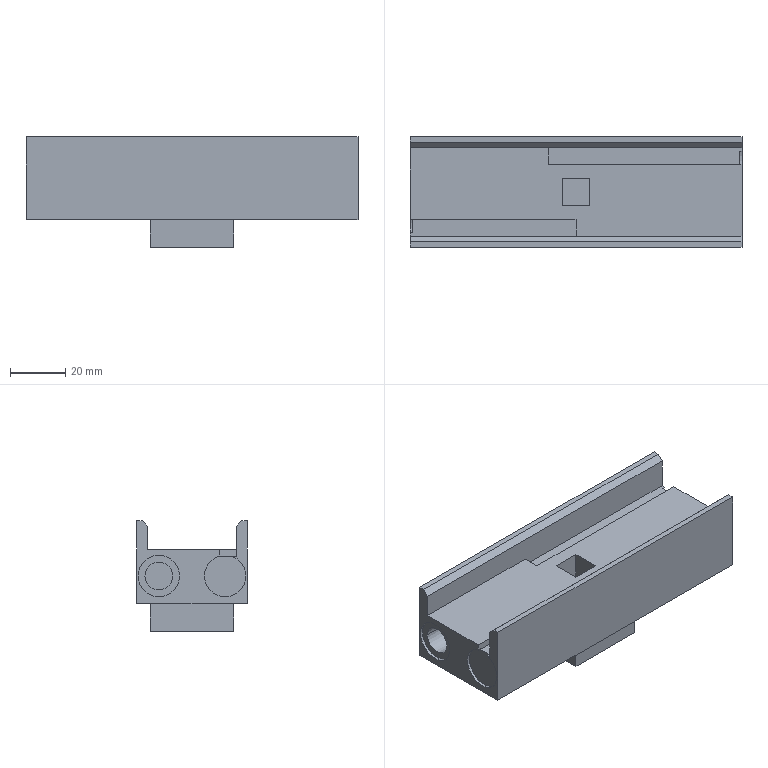Part | SolidWorks | features ICE 7, Chamfer 1, Extrusion 1, MirrorPattern 1 | 1 solid | 48 faces | box 120 x 40 x 40 mm | volume 99907 mm3 | plane 34 | cylinder 14 | commonest cylinder face diameters 15 x10 10 x4
STEP:
#1=CARTESIAN_POINT('',(-4.,17.,10.));
#2=VERTEX_POINT('',#1);
#3=CARTESIAN_POINT('',(-4.,7.,10.));
#4=VERTEX_POINT('',#3);
#5=CARTESIAN_POINT('',(-4.,12.,10.));
#6=DIRECTION('',(-1.,0.,0.));
#7=DIRECTION('',(0.,-1.,0.));
#8=AXIS2_PLACEMENT_3D('',#5,#6,#7);
#9=CIRCLE('',#8,5.);
#10=EDGE_CURVE('',#2,#4,#9,.T.);
#11=ORIENTED_EDGE('',*,*,#10,.F.);
#12=CARTESIAN_POINT('',(-59.,17.,10.));
#13=VERTEX_POINT('',#12);
#14=CARTESIAN_POINT('',(-4.,17.,10.));
#15=DIRECTION('',(-1.,0.,0.));
#16=VECTOR('',#15,1000.);
#17=LINE('',#14,#16);
#18=EDGE_CURVE('',#2,#13,#17,.T.);
#19=ORIENTED_EDGE('',*,*,#18,.T.);
#20=CARTESIAN_POINT('',(-59.,7.,10.));
#21=VERTEX_POINT('',#20);
#22=CARTESIAN_POINT('',(-59.,12.,10.));
#23=DIRECTION('',(-1.,0.,0.));
#24=DIRECTION('',(0.,-1.,0.));
#25=AXIS2_PLACEMENT_3D('',#22,#23,#24);
#26=CIRCLE('',#25,5.);
#27=EDGE_CURVE('',#13,#21,#26,.T.);
#28=ORIENTED_EDGE('',*,*,#27,.T.);
#29=CARTESIAN_POINT('',(-4.,7.,10.));
#30=DIRECTION('',(-1.,0.,0.));
#31=VECTOR('',#30,1000.);
#32=LINE('',#29,#31);
#33=EDGE_CURVE('',#4,#21,#32,.T.);
#34=ORIENTED_EDGE('',*,*,#33,.F.);
#35=EDGE_LOOP('',(#11,#19,#28,#34));
#36=FACE_OUTER_BOUND('',#35,.T.);
#37=CARTESIAN_POINT('',(-4.,12.,10.));
#38=DIRECTION('',(-1.,0.,0.));
#39=DIRECTION('',(0.,-1.,0.));
#40=AXIS2_PLACEMENT_3D('',#37,#38,#39);
#41=CYLINDRICAL_SURFACE('',#40,5.);
#42=ADVANCED_FACE('',(#36),#41,.F.);
#43=CARTESIAN_POINT('',(-59.,4.5,10.));
#44=VERTEX_POINT('',#43);
#45=CARTESIAN_POINT('',(-59.,19.5,10.));
#46=VERTEX_POINT('',#45);
#47=CARTESIAN_POINT('',(-59.,12.,10.));
#48=DIRECTION('',(1.,0.,0.));
#49=DIRECTION('',(0.,1.,0.));
#50=AXIS2_PLACEMENT_3D('',#47,#48,#49);
#51=CIRCLE('',#50,7.5);
#52=EDGE_CURVE('',#44,#46,#51,.T.);
#53=ORIENTED_EDGE('',*,*,#52,.T.);
#54=CARTESIAN_POINT('',(-60.,19.5,10.));
#55=VERTEX_POINT('',#54);
#56=CARTESIAN_POINT('',(-59.,19.5,10.));
#57=DIRECTION('',(-1.,0.,0.));
#58=VECTOR('',#57,1000.);
#59=LINE('',#56,#58);
#60=EDGE_CURVE('',#46,#55,#59,.T.);
#61=ORIENTED_EDGE('',*,*,#60,.T.);
#62=CARTESIAN_POINT('',(-60.,4.5,10.));
#63=VERTEX_POINT('',#62);
#64=CARTESIAN_POINT('',(-60.,12.,10.));
#65=DIRECTION('',(1.,0.,0.));
#66=DIRECTION('',(0.,1.,0.));
#67=AXIS2_PLACEMENT_3D('',#64,#65,#66);
#68=CIRCLE('',#67,7.5);
#69=EDGE_CURVE('',#63,#55,#68,.T.);
#70=ORIENTED_EDGE('',*,*,#69,.F.);
#71=CARTESIAN_POINT('',(-59.,4.5,10.));
#72=DIRECTION('',(-1.,0.,0.));
#73=VECTOR('',#72,1000.);
#74=LINE('',#71,#73);
#75=EDGE_CURVE('',#44,#63,#74,.T.);
#76=ORIENTED_EDGE('',*,*,#75,.F.);
#77=EDGE_LOOP('',(#53,#61,#70,#76));
#78=FACE_OUTER_BOUND('',#77,.T.);
#79=CARTESIAN_POINT('',(-59.,12.,10.));
#80=DIRECTION('',(-1.,0.,0.));
#81=DIRECTION('',(0.,-1.,0.));
#82=AXIS2_PLACEMENT_3D('',#79,#80,#81);
#83=CYLINDRICAL_SURFACE('',#82,7.5);
#84=ADVANCED_FACE('',(#78),#83,.F.);
#85=CARTESIAN_POINT('',(-59.,-19.5,10.));
#86=VERTEX_POINT('',#85);
#87=CARTESIAN_POINT('',(-59.,-4.5,10.));
#88=VERTEX_POINT('',#87);
#89=CARTESIAN_POINT('',(-59.,-12.,10.));
#90=DIRECTION('',(1.,0.,0.));
#91=DIRECTION('',(0.,1.,0.));
#92=AXIS2_PLACEMENT_3D('',#89,#90,#91);
#93=CIRCLE('',#92,7.5);
#94=EDGE_CURVE('',#86,#88,#93,.T.);
#95=ORIENTED_EDGE('',*,*,#94,.T.);
#96=CARTESIAN_POINT('',(-60.,-4.5,10.));
#97=VERTEX_POINT('',#96);
#98=CARTESIAN_POINT('',(-59.,-4.5,10.));
#99=DIRECTION('',(-1.,0.,0.));
#100=VECTOR('',#99,1000.);
#101=LINE('',#98,#100);
#102=EDGE_CURVE('',#88,#97,#101,.T.);
#103=ORIENTED_EDGE('',*,*,#102,.T.);
#104=CARTESIAN_POINT('',(-60.,-19.5,10.));
#105=VERTEX_POINT('',#104);
#106=CARTESIAN_POINT('',(-60.,-12.,10.));
#107=DIRECTION('',(1.,0.,0.));
#108=DIRECTION('',(0.,1.,0.));
#109=AXIS2_PLACEMENT_3D('',#106,#107,#108);
#110=CIRCLE('',#109,7.5);
#111=EDGE_CURVE('',#105,#97,#110,.T.);
#112=ORIENTED_EDGE('',*,*,#111,.F.);
#113=CARTESIAN_POINT('',(-59.,-19.5,10.));
#114=DIRECTION('',(-1.,0.,0.));
#115=VECTOR('',#114,1000.);
#116=LINE('',#113,#115);
#117=EDGE_CURVE('',#86,#105,#116,.T.);
#118=ORIENTED_EDGE('',*,*,#117,.F.);
#119=EDGE_LOOP('',(#95,#103,#112,#118));
#120=FACE_OUTER_BOUND('',#119,.T.);
#121=CARTESIAN_POINT('',(-59.,-12.,10.));
#122=DIRECTION('',(-1.,0.,0.));
#123=DIRECTION('',(0.,-1.,0.));
#124=AXIS2_PLACEMENT_3D('',#121,#122,#123);
#125=CYLINDRICAL_SURFACE('',#124,7.5);
#126=ADVANCED_FACE('',(#120),#125,.F.);
#127=CARTESIAN_POINT('',(-59.,-14.693,17.));
#128=VERTEX_POINT('',#127);
#129=CARTESIAN_POINT('',(-59.,-12.,10.));
#130=DIRECTION('',(1.,0.,0.));
#131=DIRECTION('',(0.,1.,0.));
#132=AXIS2_PLACEMENT_3D('',#129,#130,#131);
#133=CIRCLE('',#132,7.5);
#134=EDGE_CURVE('',#128,#86,#133,.T.);
#135=ORIENTED_EDGE('',*,*,#134,.T.);
#136=ORIENTED_EDGE('',*,*,#117,.T.);
#137=CARTESIAN_POINT('',(-60.,-14.693,17.));
#138=VERTEX_POINT('',#137);
#139=CARTESIAN_POINT('',(-60.,-12.,10.));
#140=DIRECTION('',(1.,0.,0.));
#141=DIRECTION('',(0.,1.,0.));
#142=AXIS2_PLACEMENT_3D('',#139,#140,#141);
#143=CIRCLE('',#142,7.5);
#144=EDGE_CURVE('',#138,#105,#143,.T.);
#145=ORIENTED_EDGE('',*,*,#144,.F.);
#146=CARTESIAN_POINT('',(-59.,-14.693,17.));
#147=DIRECTION('',(1.,0.,0.));
#148=VECTOR('',#147,1000.);
#149=LINE('',#146,#148);
#150=EDGE_CURVE('',#138,#128,#149,.T.);
#151=ORIENTED_EDGE('',*,*,#150,.T.);
#152=EDGE_LOOP('',(#135,#136,#145,#151));
#153=FACE_OUTER_BOUND('',#152,.T.);
#154=CARTESIAN_POINT('',(-59.,-12.,10.));
#155=DIRECTION('',(-1.,0.,0.));
#156=DIRECTION('',(0.,-1.,0.));
#157=AXIS2_PLACEMENT_3D('',#154,#155,#156);
#158=CYLINDRICAL_SURFACE('',#157,7.5);
#159=ADVANCED_FACE('',(#153),#158,.F.);
#160=CARTESIAN_POINT('',(4.,-17.,10.));
#161=VERTEX_POINT('',#160);
#162=CARTESIAN_POINT('',(4.,-7.,10.));
#163=VERTEX_POINT('',#162);
#164=CARTESIAN_POINT('',(4.,-12.,10.));
#165=DIRECTION('',(1.,0.,0.));
#166=DIRECTION('',(0.,1.,0.));
#167=AXIS2_PLACEMENT_3D('',#164,#165,#166);
#168=CIRCLE('',#167,5.);
#169=EDGE_CURVE('',#161,#163,#168,.T.);
#170=ORIENTED_EDGE('',*,*,#169,.F.);
#171=CARTESIAN_POINT('',(59.,-17.,10.));
#172=VERTEX_POINT('',#171);
#173=CARTESIAN_POINT('',(4.,-17.,10.));
#174=DIRECTION('',(1.,0.,0.));
#175=VECTOR('',#174,1000.);
#176=LINE('',#173,#175);
#177=EDGE_CURVE('',#161,#172,#176,.T.);
#178=ORIENTED_EDGE('',*,*,#177,.T.);
#179=CARTESIAN_POINT('',(59.,-7.,10.));
#180=VERTEX_POINT('',#179);
#181=CARTESIAN_POINT('',(59.,-12.,10.));
#182=DIRECTION('',(1.,0.,0.));
#183=DIRECTION('',(0.,1.,0.));
#184=AXIS2_PLACEMENT_3D('',#181,#182,#183);
#185=CIRCLE('',#184,5.);
#186=EDGE_CURVE('',#172,#180,#185,.T.);
#187=ORIENTED_EDGE('',*,*,#186,.T.);
#188=CARTESIAN_POINT('',(4.,-7.,10.));
#189=DIRECTION('',(1.,0.,0.));
#190=VECTOR('',#189,1000.);
#191=LINE('',#188,#190);
#192=EDGE_CURVE('',#163,#180,#191,.T.);
#193=ORIENTED_EDGE('',*,*,#192,.F.);
#194=EDGE_LOOP('',(#170,#178,#187,#193));
#195=FACE_OUTER_BOUND('',#194,.T.);
#196=CARTESIAN_POINT('',(4.,-12.,10.));
#197=DIRECTION('',(1.,0.,0.));
#198=DIRECTION('',(0.,1.,0.));
#199=AXIS2_PLACEMENT_3D('',#196,#197,#198);
#200=CYLINDRICAL_SURFACE('',#199,5.);
#201=ADVANCED_FACE('',(#195),#200,.F.);
#202=CARTESIAN_POINT('',(59.,4.5,10.));
#203=VERTEX_POINT('',#202);
#204=CARTESIAN_POINT('',(59.,19.5,10.));
#205=VERTEX_POINT('',#204);
#206=CARTESIAN_POINT('',(59.,12.,10.));
#207=DIRECTION('',(1.,0.,0.));
#208=DIRECTION('',(0.,1.,0.));
#209=AXIS2_PLACEMENT_3D('',#206,#207,#208);
#210=CIRCLE('',#209,7.5);
#211=EDGE_CURVE('',#203,#205,#210,.T.);
#212=ORIENTED_EDGE('',*,*,#211,.F.);
#213=CARTESIAN_POINT('',(60.,4.5,10.));
#214=VERTEX_POINT('',#213);
#215=CARTESIAN_POINT('',(59.,4.5,10.));
#216=DIRECTION('',(1.,0.,0.));
#217=VECTOR('',#216,1000.);
#218=LINE('',#215,#217);
#219=EDGE_CURVE('',#203,#214,#218,.T.);
#220=ORIENTED_EDGE('',*,*,#219,.T.);
#221=CARTESIAN_POINT('',(60.,19.5,10.));
#222=VERTEX_POINT('',#221);
#223=CARTESIAN_POINT('',(60.,12.,10.));
#224=DIRECTION('',(1.,0.,0.));
#225=DIRECTION('',(0.,1.,0.));
#226=AXIS2_PLACEMENT_3D('',#223,#224,#225);
#227=CIRCLE('',#226,7.5);
#228=EDGE_CURVE('',#214,#222,#227,.T.);
#229=ORIENTED_EDGE('',*,*,#228,.T.);
#230=CARTESIAN_POINT('',(59.,19.5,10.));
#231=DIRECTION('',(1.,0.,0.));
#232=VECTOR('',#231,1000.);
#233=LINE('',#230,#232);
#234=EDGE_CURVE('',#205,#222,#233,.T.);
#235=ORIENTED_EDGE('',*,*,#234,.F.);
#236=EDGE_LOOP('',(#212,#220,#229,#235));
#237=FACE_OUTER_BOUND('',#236,.T.);
#238=CARTESIAN_POINT('',(59.,12.,10.));
#239=DIRECTION('',(1.,0.,0.));
#240=DIRECTION('',(0.,1.,0.));
#241=AXIS2_PLACEMENT_3D('',#238,#239,#240);
#242=CYLINDRICAL_SURFACE('',#241,7.5);
#243=ADVANCED_FACE('',(#237),#242,.F.);
#244=CARTESIAN_POINT('',(59.,14.693,17.));
#245=VERTEX_POINT('',#244);
#246=CARTESIAN_POINT('',(59.,12.,10.));
#247=DIRECTION('',(1.,0.,0.));
#248=DIRECTION('',(0.,1.,0.));
#249=AXIS2_PLACEMENT_3D('',#246,#247,#248);
#250=CIRCLE('',#249,7.5);
#251=EDGE_CURVE('',#205,#245,#250,.T.);
#252=ORIENTED_EDGE('',*,*,#251,.F.);
#253=ORIENTED_EDGE('',*,*,#234,.T.);
#254=CARTESIAN_POINT('',(60.,14.693,17.));
#255=VERTEX_POINT('',#254);
#256=CARTESIAN_POINT('',(60.,12.,10.));
#257=DIRECTION('',(1.,0.,0.));
#258=DIRECTION('',(0.,1.,0.));
#259=AXIS2_PLACEMENT_3D('',#256,#257,#258);
#260=CIRCLE('',#259,7.5);
#261=EDGE_CURVE('',#222,#255,#260,.T.);
#262=ORIENTED_EDGE('',*,*,#261,.T.);
#263=CARTESIAN_POINT('',(59.,14.693,17.));
#264=DIRECTION('',(1.,0.,0.));
#265=VECTOR('',#264,1000.);
#266=LINE('',#263,#265);
#267=EDGE_CURVE('',#245,#255,#266,.T.);
#268=ORIENTED_EDGE('',*,*,#267,.F.);
#269=EDGE_LOOP('',(#252,#253,#262,#268));
#270=FACE_OUTER_BOUND('',#269,.T.);
#271=CARTESIAN_POINT('',(59.,12.,10.));
#272=DIRECTION('',(1.,0.,0.));
#273=DIRECTION('',(0.,1.,0.));
#274=AXIS2_PLACEMENT_3D('',#271,#272,#273);
#275=CYLINDRICAL_SURFACE('',#274,7.5);
#276=ADVANCED_FACE('',(#270),#275,.F.);
#277=CARTESIAN_POINT('',(59.,-19.5,10.));
#278=VERTEX_POINT('',#277);
#279=CARTESIAN_POINT('',(59.,-4.5,10.));
#280=VERTEX_POINT('',#279);
#281=CARTESIAN_POINT('',(59.,-12.,10.));
#282=DIRECTION('',(1.,0.,0.));
#283=DIRECTION('',(0.,1.,0.));
#284=AXIS2_PLACEMENT_3D('',#281,#282,#283);
#285=CIRCLE('',#284,7.5);
#286=EDGE_CURVE('',#278,#280,#285,.T.);
#287=ORIENTED_EDGE('',*,*,#286,.F.);
#288=CARTESIAN_POINT('',(60.,-19.5,10.));
#289=VERTEX_POINT('',#288);
#290=CARTESIAN_POINT('',(59.,-19.5,10.));
#291=DIRECTION('',(1.,0.,0.));
#292=VECTOR('',#291,1000.);
#293=LINE('',#290,#292);
#294=EDGE_CURVE('',#278,#289,#293,.T.);
#295=ORIENTED_EDGE('',*,*,#294,.T.);
#296=CARTESIAN_POINT('',(60.,-4.5,10.));
#297=VERTEX_POINT('',#296);
#298=CARTESIAN_POINT('',(60.,-12.,10.));
#299=DIRECTION('',(1.,0.,0.));
#300=DIRECTION('',(0.,1.,0.));
#301=AXIS2_PLACEMENT_3D('',#298,#299,#300);
#302=CIRCLE('',#301,7.5);
#303=EDGE_CURVE('',#289,#297,#302,.T.);
#304=ORIENTED_EDGE('',*,*,#303,.T.);
#305=CARTESIAN_POINT('',(59.,-4.5,10.));
#306=DIRECTION('',(1.,0.,0.));
#307=VECTOR('',#306,1000.);
#308=LINE('',#305,#307);
#309=EDGE_CURVE('',#280,#297,#308,.T.);
#310=ORIENTED_EDGE('',*,*,#309,.F.);
#311=EDGE_LOOP('',(#287,#295,#304,#310));
#312=FACE_OUTER_BOUND('',#311,.T.);
#313=CARTESIAN_POINT('',(59.,-12.,10.));
#314=DIRECTION('',(1.,0.,0.));
#315=DIRECTION('',(0.,1.,0.));
#316=AXIS2_PLACEMENT_3D('',#313,#314,#315);
#317=CYLINDRICAL_SURFACE('',#316,7.5);
#318=ADVANCED_FACE('',(#312),#317,.F.);
#319=ORIENTED_EDGE('',*,*,#150,.F.);
#320=CARTESIAN_POINT('',(-60.,-16.,17.));
#321=VERTEX_POINT('',#320);
#322=CARTESIAN_POINT('',(-60.,-16.,17.));
#323=DIRECTION('',(0.,-1.,0.));
#324=VECTOR('',#323,1000.);
#325=LINE('',#322,#324);
#326=EDGE_CURVE('',#138,#321,#325,.T.);
#327=ORIENTED_EDGE('',*,*,#326,.T.);
#328=CARTESIAN_POINT('',(0.,-16.,17.));
#329=VERTEX_POINT('',#328);
#330=CARTESIAN_POINT('',(0.,-16.,17.));
#331=DIRECTION('',(-1.,0.,0.));
#332=VECTOR('',#331,1000.);
#333=LINE('',#330,#332);
#334=EDGE_CURVE('',#329,#321,#333,.T.);
#335=ORIENTED_EDGE('',*,*,#334,.F.);
#336=CARTESIAN_POINT('',(0.,-10.,17.));
#337=VERTEX_POINT('',#336);
#338=CARTESIAN_POINT('',(0.,-16.,17.));
#339=DIRECTION('',(0.,-1.,0.));
#340=VECTOR('',#339,1000.);
#341=LINE('',#338,#340);
#342=EDGE_CURVE('',#337,#329,#341,.T.);
#343=ORIENTED_EDGE('',*,*,#342,.F.);
#344=CARTESIAN_POINT('',(-59.,-10.,17.));
#345=VERTEX_POINT('',#344);
#346=CARTESIAN_POINT('',(0.,-10.,17.));
#347=DIRECTION('',(-1.,0.,0.));
#348=VECTOR('',#347,1000.);
#349=LINE('',#346,#348);
#350=EDGE_CURVE('',#337,#345,#349,.T.);
#351=ORIENTED_EDGE('',*,*,#350,.T.);
#352=CARTESIAN_POINT('',(-59.,-16.,17.));
#353=DIRECTION('',(0.,1.,0.));
#354=VECTOR('',#353,1000.);
#355=LINE('',#352,#354);
#356=EDGE_CURVE('',#128,#345,#355,.T.);
#357=ORIENTED_EDGE('',*,*,#356,.F.);
#358=EDGE_LOOP('',(#319,#327,#335,#343,#351,#357));
#359=FACE_OUTER_BOUND('',#358,.T.);
#360=CARTESIAN_POINT('',(0.,-16.,17.));
#361=DIRECTION('',(0.,0.,-1.));
#362=DIRECTION('',(-1.,0.,0.));
#363=AXIS2_PLACEMENT_3D('',#360,#361,#362);
#364=PLANE('',#363);
#365=ADVANCED_FACE('',(#359),#364,.F.);
#366=CARTESIAN_POINT('',(-59.,-10.,17.228));
#367=VERTEX_POINT('',#366);
#368=CARTESIAN_POINT('',(-60.,-10.,17.228));
#369=VERTEX_POINT('',#368);
#370=CARTESIAN_POINT('',(-59.,-10.,17.228));
#371=DIRECTION('',(-1.,0.,0.));
#372=VECTOR('',#371,1000.);
#373=LINE('',#370,#372);
#374=EDGE_CURVE('',#367,#369,#373,.T.);
#375=ORIENTED_EDGE('',*,*,#374,.F.);
#376=CARTESIAN_POINT('',(-59.,-10.,19.5));
#377=DIRECTION('',(0.,0.,1.));
#378=VECTOR('',#377,1000.);
#379=LINE('',#376,#378);
#380=EDGE_CURVE('',#345,#367,#379,.T.);
#381=ORIENTED_EDGE('',*,*,#380,.F.);
#382=ORIENTED_EDGE('',*,*,#350,.F.);
#383=CARTESIAN_POINT('',(0.,-10.,19.5));
#384=VERTEX_POINT('',#383);
#385=CARTESIAN_POINT('',(0.,-10.,19.5));
#386=DIRECTION('',(0.,0.,-1.));
#387=VECTOR('',#386,1000.);
#388=LINE('',#385,#387);
#389=EDGE_CURVE('',#384,#337,#388,.T.);
#390=ORIENTED_EDGE('',*,*,#389,.F.);
#391=CARTESIAN_POINT('',(-60.,-10.,19.5));
#392=VERTEX_POINT('',#391);
#393=CARTESIAN_POINT('',(0.,-10.,19.5));
#394=DIRECTION('',(-1.,0.,0.));
#395=VECTOR('',#394,1000.);
#396=LINE('',#393,#395);
#397=EDGE_CURVE('',#384,#392,#396,.T.);
#398=ORIENTED_EDGE('',*,*,#397,.T.);
#399=CARTESIAN_POINT('',(-60.,-10.,19.5));
#400=DIRECTION('',(0.,0.,-1.));
#401=VECTOR('',#400,1000.);
#402=LINE('',#399,#401);
#403=EDGE_CURVE('',#392,#369,#402,.T.);
#404=ORIENTED_EDGE('',*,*,#403,.T.);
#405=EDGE_LOOP('',(#375,#381,#382,#390,#398,#404));
#406=FACE_OUTER_BOUND('',#405,.T.);
#407=CARTESIAN_POINT('',(0.,-10.,19.5));
#408=DIRECTION('',(0.,1.,0.));
#409=DIRECTION('',(-1.,0.,0.));
#410=AXIS2_PLACEMENT_3D('',#407,#408,#409);
#411=PLANE('',#410);
#412=ADVANCED_FACE('',(#406),#411,.F.);
#413=CARTESIAN_POINT('',(60.,-20.,0.));
#414=VERTEX_POINT('',#413);
#415=CARTESIAN_POINT('',(60.,20.,0.));
#416=VERTEX_POINT('',#415);
#417=CARTESIAN_POINT('',(60.,20.,0.));
#418=DIRECTION('',(0.,1.,0.));
#419=VECTOR('',#418,1000.);
#420=LINE('',#417,#419);
#421=EDGE_CURVE('',#414,#416,#420,.T.);
#422=ORIENTED_EDGE('',*,*,#421,.F.);
#423=CARTESIAN_POINT('',(-60.,-20.,0.));
#424=VERTEX_POINT('',#423);
#425=CARTESIAN_POINT('',(-60.,-20.,0.));
#426=DIRECTION('',(1.,0.,0.));
#427=VECTOR('',#426,1000.);
#428=LINE('',#425,#427);
#429=EDGE_CURVE('',#424,#414,#428,.T.);
#430=ORIENTED_EDGE('',*,*,#429,.F.);
#431=CARTESIAN_POINT('',(-60.,20.,0.));
#432=VERTEX_POINT('',#431);
#433=CARTESIAN_POINT('',(-60.,20.,0.));
#434=DIRECTION('',(0.,-1.,0.));
#435=VECTOR('',#434,1000.);
#436=LINE('',#433,#435);
#437=EDGE_CURVE('',#432,#424,#436,.T.);
#438=ORIENTED_EDGE('',*,*,#437,.F.);
#439=CARTESIAN_POINT('',(-60.,20.,0.));
#440=DIRECTION('',(-1.,0.,0.));
#441=VECTOR('',#440,1000.);
#442=LINE('',#439,#441);
#443=EDGE_CURVE('',#416,#432,#442,.T.);
#444=ORIENTED_EDGE('',*,*,#443,.F.);
#445=EDGE_LOOP('',(#422,#430,#438,#444));
#446=FACE_OUTER_BOUND('',#445,.T.);
#447=CARTESIAN_POINT('',(-15.,-15.,0.));
#448=VERTEX_POINT('',#447);
#449=CARTESIAN_POINT('',(-15.,15.,0.));
#450=VERTEX_POINT('',#449);
#451=CARTESIAN_POINT('',(-15.,15.,0.));
#452=DIRECTION('',(0.,1.,0.));
#453=VECTOR('',#452,1000.);
#454=LINE('',#451,#453);
#455=EDGE_CURVE('',#448,#450,#454,.T.);
#456=ORIENTED_EDGE('',*,*,#455,.F.);
#457=CARTESIAN_POINT('',(15.,-15.,0.));
#458=VERTEX_POINT('',#457);
#459=CARTESIAN_POINT('',(15.,-15.,0.));
#460=DIRECTION('',(-1.,0.,0.));
#461=VECTOR('',#460,1000.);
#462=LINE('',#459,#461);
#463=EDGE_CURVE('',#458,#448,#462,.T.);
#464=ORIENTED_EDGE('',*,*,#463,.F.);
#465=CARTESIAN_POINT('',(15.,15.,0.));
#466=VERTEX_POINT('',#465);
#467=CARTESIAN_POINT('',(15.,15.,0.));
#468=DIRECTION('',(0.,-1.,0.));
#469=VECTOR('',#468,1000.);
#470=LINE('',#467,#469);
#471=EDGE_CURVE('',#466,#458,#470,.T.);
#472=ORIENTED_EDGE('',*,*,#471,.F.);
#473=CARTESIAN_POINT('',(15.,15.,0.));
#474=DIRECTION('',(1.,0.,0.));
#475=VECTOR('',#474,1000.);
#476=LINE('',#473,#475);
#477=EDGE_CURVE('',#450,#466,#476,.T.);
#478=ORIENTED_EDGE('',*,*,#477,.F.);
#479=EDGE_LOOP('',(#456,#464,#472,#478));
#480=FACE_BOUND('',#479,.T.);
#481=CARTESIAN_POINT('',(0.,0.,0.));
#482=DIRECTION('',(0.,0.,1.));
#483=DIRECTION('',(1.,0.,0.));
#484=AXIS2_PLACEMENT_3D('',#481,#482,#483);
#485=PLANE('',#484);
#486=ADVANCED_FACE('',(#446,#480),#485,.F.);
#487=CARTESIAN_POINT('',(60.,-20.,30.));
#488=VERTEX_POINT('',#487);
#489=CARTESIAN_POINT('',(60.,-18.,30.));
#490=VERTEX_POINT('',#489);
#491=CARTESIAN_POINT('',(60.,20.,30.));
#492=DIRECTION('',(0.,1.,0.));
#493=VECTOR('',#492,1000.);
#494=LINE('',#491,#493);
#495=EDGE_CURVE('',#488,#490,#494,.T.);
#496=ORIENTED_EDGE('',*,*,#495,.T.);
#497=CARTESIAN_POINT('',(-60.,-18.,30.));
#498=VERTEX_POINT('',#497);
#499=CARTESIAN_POINT('',(-60.,-18.,30.));
#500=DIRECTION('',(-1.,0.,0.));
#501=VECTOR('',#500,1000.);
#502=LINE('',#499,#501);
#503=EDGE_CURVE('',#490,#498,#502,.T.);
#504=ORIENTED_EDGE('',*,*,#503,.T.);
#505=CARTESIAN_POINT('',(-60.,-20.,30.));
#506=VERTEX_POINT('',#505);
#507=CARTESIAN_POINT('',(-60.,20.,30.));
#508=DIRECTION('',(0.,-1.,0.));
#509=VECTOR('',#508,1000.);
#510=LINE('',#507,#509);
#511=EDGE_CURVE('',#498,#506,#510,.T.);
#512=ORIENTED_EDGE('',*,*,#511,.T.);
#513=CARTESIAN_POINT('',(-60.,-20.,30.));
#514=DIRECTION('',(1.,0.,0.));
#515=VECTOR('',#514,1000.);
#516=LINE('',#513,#515);
#517=EDGE_CURVE('',#506,#488,#516,.T.);
#518=ORIENTED_EDGE('',*,*,#517,.T.);
#519=EDGE_LOOP('',(#496,#504,#512,#518));
#520=FACE_OUTER_BOUND('',#519,.T.);
#521=CARTESIAN_POINT('',(0.,0.,30.));
#522=DIRECTION('',(0.,0.,1.));
#523=DIRECTION('',(1.,0.,0.));
#524=AXIS2_PLACEMENT_3D('',#521,#522,#523);
#525=PLANE('',#524);
#526=ADVANCED_FACE('',(#520),#525,.T.);
#527=CARTESIAN_POINT('',(60.,-12.,10.));
#528=DIRECTION('',(1.,0.,0.));
#529=DIRECTION('',(0.,1.,0.));
#530=AXIS2_PLACEMENT_3D('',#527,#528,#529);
#531=CIRCLE('',#530,7.5);
#532=EDGE_CURVE('',#297,#289,#531,.T.);
#533=ORIENTED_EDGE('',*,*,#532,.F.);
#534=ORIENTED_EDGE('',*,*,#303,.F.);
#535=EDGE_LOOP('',(#533,#534));
#536=FACE_BOUND('',#535,.T.);
#537=CARTESIAN_POINT('',(60.,16.,17.));
#538=VERTEX_POINT('',#537);
#539=CARTESIAN_POINT('',(60.,16.,17.));
#540=DIRECTION('',(0.,1.,0.));
#541=VECTOR('',#540,1000.);
#542=LINE('',#539,#541);
#543=EDGE_CURVE('',#255,#538,#542,.T.);
#544=ORIENTED_EDGE('',*,*,#543,.F.);
#545=ORIENTED_EDGE('',*,*,#261,.F.);
#546=ORIENTED_EDGE('',*,*,#228,.F.);
#547=CARTESIAN_POINT('',(60.,10.,17.228));
#548=VERTEX_POINT('',#547);
#549=CARTESIAN_POINT('',(60.,12.,10.));
#550=DIRECTION('',(1.,0.,0.));
#551=DIRECTION('',(0.,1.,0.));
#552=AXIS2_PLACEMENT_3D('',#549,#550,#551);
#553=CIRCLE('',#552,7.5);
#554=EDGE_CURVE('',#548,#214,#553,.T.);
#555=ORIENTED_EDGE('',*,*,#554,.F.);
#556=CARTESIAN_POINT('',(60.,10.,19.5));
#557=VERTEX_POINT('',#556);
#558=CARTESIAN_POINT('',(60.,10.,19.5));
#559=DIRECTION('',(0.,0.,-1.));
#560=VECTOR('',#559,1000.);
#561=LINE('',#558,#560);
#562=EDGE_CURVE('',#557,#548,#561,.T.);
#563=ORIENTED_EDGE('',*,*,#562,.F.);
#564=CARTESIAN_POINT('',(60.,-16.,19.5));
#565=VERTEX_POINT('',#564);
#566=CARTESIAN_POINT('',(60.,10.,19.5));
#567=DIRECTION('',(0.,1.,0.));
#568=VECTOR('',#567,1000.);
#569=LINE('',#566,#568);
#570=EDGE_CURVE('',#565,#557,#569,.T.);
#571=ORIENTED_EDGE('',*,*,#570,.F.);
#572=CARTESIAN_POINT('',(60.,-16.,28.));
#573=VERTEX_POINT('',#572);
#574=CARTESIAN_POINT('',(60.,-16.,30.));
#575=DIRECTION('',(0.,0.,-1.));
#576=VECTOR('',#575,1000.);
#577=LINE('',#574,#576);
#578=EDGE_CURVE('',#573,#565,#577,.T.);
#579=ORIENTED_EDGE('',*,*,#578,.F.);
#580=CARTESIAN_POINT('',(60.,-16.,28.));
#581=DIRECTION('',(0.,-0.7071,0.7071));
#582=VECTOR('',#581,1000.);
#583=LINE('',#580,#582);
#584=EDGE_CURVE('',#573,#490,#583,.T.);
#585=ORIENTED_EDGE('',*,*,#584,.T.);
#586=ORIENTED_EDGE('',*,*,#495,.F.);
#587=CARTESIAN_POINT('',(60.,-20.,30.));
#588=DIRECTION('',(0.,0.,-1.));
#589=VECTOR('',#588,1000.);
#590=LINE('',#587,#589);
#591=EDGE_CURVE('',#488,#414,#590,.T.);
#592=ORIENTED_EDGE('',*,*,#591,.T.);
#593=ORIENTED_EDGE('',*,*,#421,.T.);
#594=CARTESIAN_POINT('',(60.,20.,30.));
#595=VERTEX_POINT('',#594);
#596=CARTESIAN_POINT('',(60.,20.,30.));
#597=DIRECTION('',(0.,0.,-1.));
#598=VECTOR('',#597,1000.);
#599=LINE('',#596,#598);
#600=EDGE_CURVE('',#595,#416,#599,.T.);
#601=ORIENTED_EDGE('',*,*,#600,.F.);
#602=CARTESIAN_POINT('',(60.,18.,30.));
#603=VERTEX_POINT('',#602);
#604=CARTESIAN_POINT('',(60.,20.,30.));
#605=DIRECTION('',(0.,1.,0.));
#606=VECTOR('',#605,1000.);
#607=LINE('',#604,#606);
#608=EDGE_CURVE('',#603,#595,#607,.T.);
#609=ORIENTED_EDGE('',*,*,#608,.F.);
#610=CARTESIAN_POINT('',(60.,16.,28.));
#611=VERTEX_POINT('',#610);
#612=CARTESIAN_POINT('',(60.,18.,30.));
#613=DIRECTION('',(0.,-0.7071,-0.7071));
#614=VECTOR('',#613,1000.);
#615=LINE('',#612,#614);
#616=EDGE_CURVE('',#603,#611,#615,.T.);
#617=ORIENTED_EDGE('',*,*,#616,.T.);
#618=CARTESIAN_POINT('',(60.,16.,30.));
#619=DIRECTION('',(0.,0.,1.));
#620=VECTOR('',#619,1000.);
#621=LINE('',#618,#620);
#622=EDGE_CURVE('',#538,#611,#621,.T.);
#623=ORIENTED_EDGE('',*,*,#622,.F.);
#624=EDGE_LOOP('',(#544,#545,#546,#555,#563,#571,#579,#585,#586,#592,#593,#601,#609,#617,#623));
#625=FACE_OUTER_BOUND('',#624,.T.);
#626=CARTESIAN_POINT('',(60.,20.,30.));
#627=DIRECTION('',(-1.,0.,0.));
#628=DIRECTION('',(0.,-1.,0.));
#629=AXIS2_PLACEMENT_3D('',#626,#627,#628);
#630=PLANE('',#629);
#631=ADVANCED_FACE('',(#536,#625),#630,.F.);
#632=ORIENTED_EDGE('',*,*,#443,.T.);
#633=CARTESIAN_POINT('',(-60.,20.,30.));
#634=VERTEX_POINT('',#633);
#635=CARTESIAN_POINT('',(-60.,20.,30.));
#636=DIRECTION('',(0.,0.,-1.));
#637=VECTOR('',#636,1000.);
#638=LINE('',#635,#637);
#639=EDGE_CURVE('',#634,#432,#638,.T.);
#640=ORIENTED_EDGE('',*,*,#639,.F.);
#641=CARTESIAN_POINT('',(-60.,20.,30.));
#642=DIRECTION('',(-1.,0.,0.));
#643=VECTOR('',#642,1000.);
#644=LINE('',#641,#643);
#645=EDGE_CURVE('',#595,#634,#644,.T.);
#646=ORIENTED_EDGE('',*,*,#645,.F.);
#647=ORIENTED_EDGE('',*,*,#600,.T.);
#648=EDGE_LOOP('',(#632,#640,#646,#647));
#649=FACE_OUTER_BOUND('',#648,.T.);
#650=CARTESIAN_POINT('',(-60.,20.,30.));
#651=DIRECTION('',(0.,-1.,0.));
#652=DIRECTION('',(0.,0.,-1.));
#653=AXIS2_PLACEMENT_3D('',#650,#651,#652);
#654=PLANE('',#653);
#655=ADVANCED_FACE('',(#649),#654,.F.);
#656=ORIENTED_EDGE('',*,*,#69,.T.);
#657=CARTESIAN_POINT('',(-60.,12.,10.));
#658=DIRECTION('',(1.,0.,0.));
#659=DIRECTION('',(0.,1.,0.));
#660=AXIS2_PLACEMENT_3D('',#657,#658,#659);
#661=CIRCLE('',#660,7.5);
#662=EDGE_CURVE('',#55,#63,#661,.T.);
#663=ORIENTED_EDGE('',*,*,#662,.T.);
#664=EDGE_LOOP('',(#656,#663));
#665=FACE_BOUND('',#664,.T.);
#666=ORIENTED_EDGE('',*,*,#144,.T.);
#667=ORIENTED_EDGE('',*,*,#111,.T.);
#668=CARTESIAN_POINT('',(-60.,-12.,10.));
#669=DIRECTION('',(1.,0.,0.));
#670=DIRECTION('',(0.,1.,0.));
#671=AXIS2_PLACEMENT_3D('',#668,#669,#670);
#672=CIRCLE('',#671,7.5);
#673=EDGE_CURVE('',#97,#369,#672,.T.);
#674=ORIENTED_EDGE('',*,*,#673,.T.);
#675=ORIENTED_EDGE('',*,*,#403,.F.);
#676=CARTESIAN_POINT('',(-60.,16.,19.5));
#677=VERTEX_POINT('',#676);
#678=CARTESIAN_POINT('',(-60.,16.,19.5));
#679=DIRECTION('',(0.,-1.,0.));
#680=VECTOR('',#679,1000.);
#681=LINE('',#678,#680);
#682=EDGE_CURVE('',#677,#392,#681,.T.);
#683=ORIENTED_EDGE('',*,*,#682,.F.);
#684=CARTESIAN_POINT('',(-60.,16.,28.));
#685=VERTEX_POINT('',#684);
#686=CARTESIAN_POINT('',(-60.,16.,30.));
#687=DIRECTION('',(0.,0.,-1.));
#688=VECTOR('',#687,1000.);
#689=LINE('',#686,#688);
#690=EDGE_CURVE('',#685,#677,#689,.T.);
#691=ORIENTED_EDGE('',*,*,#690,.F.);
#692=CARTESIAN_POINT('',(-60.,18.,30.));
#693=VERTEX_POINT('',#692);
#694=CARTESIAN_POINT('',(-60.,18.,30.));
#695=DIRECTION('',(0.,0.7071,0.7071));
#696=VECTOR('',#695,1000.);
#697=LINE('',#694,#696);
#698=EDGE_CURVE('',#685,#693,#697,.T.);
#699=ORIENTED_EDGE('',*,*,#698,.T.);
#700=CARTESIAN_POINT('',(-60.,20.,30.));
#701=DIRECTION('',(0.,-1.,0.));
#702=VECTOR('',#701,1000.);
#703=LINE('',#700,#702);
#704=EDGE_CURVE('',#634,#693,#703,.T.);
#705=ORIENTED_EDGE('',*,*,#704,.F.);
#706=ORIENTED_EDGE('',*,*,#639,.T.);
#707=ORIENTED_EDGE('',*,*,#437,.T.);
#708=CARTESIAN_POINT('',(-60.,-20.,30.));
#709=DIRECTION('',(0.,0.,-1.));
#710=VECTOR('',#709,1000.);
#711=LINE('',#708,#710);
#712=EDGE_CURVE('',#506,#424,#711,.T.);
#713=ORIENTED_EDGE('',*,*,#712,.F.);
#714=ORIENTED_EDGE('',*,*,#511,.F.);
#715=CARTESIAN_POINT('',(-60.,-16.,28.));
#716=VERTEX_POINT('',#715);
#717=CARTESIAN_POINT('',(-60.,-16.,28.));
#718=DIRECTION('',(0.,0.7071,-0.7071));
#719=VECTOR('',#718,1000.);
#720=LINE('',#717,#719);
#721=EDGE_CURVE('',#498,#716,#720,.T.);
#722=ORIENTED_EDGE('',*,*,#721,.T.);
#723=CARTESIAN_POINT('',(-60.,-16.,30.));
#724=DIRECTION('',(0.,0.,1.));
#725=VECTOR('',#724,1000.);
#726=LINE('',#723,#725);
#727=EDGE_CURVE('',#321,#716,#726,.T.);
#728=ORIENTED_EDGE('',*,*,#727,.F.);
#729=ORIENTED_EDGE('',*,*,#326,.F.);
#730=EDGE_LOOP('',(#666,#667,#674,#675,#683,#691,#699,#705,#706,#707,#713,#714,#722,#728,#729));
#731=FACE_OUTER_BOUND('',#730,.T.);
#732=CARTESIAN_POINT('',(-60.,20.,30.));
#733=DIRECTION('',(1.,0.,0.));
#734=DIRECTION('',(0.,1.,0.));
#735=AXIS2_PLACEMENT_3D('',#732,#733,#734);
#736=PLANE('',#735);
#737=ADVANCED_FACE('',(#665,#731),#736,.F.);
#738=ORIENTED_EDGE('',*,*,#429,.T.);
#739=ORIENTED_EDGE('',*,*,#591,.F.);
#740=ORIENTED_EDGE('',*,*,#517,.F.);
#741=ORIENTED_EDGE('',*,*,#712,.T.);
#742=EDGE_LOOP('',(#738,#739,#740,#741));
#743=FACE_OUTER_BOUND('',#742,.T.);
#744=CARTESIAN_POINT('',(-60.,-20.,30.));
#745=DIRECTION('',(0.,1.,0.));
#746=DIRECTION('',(0.,0.,1.));
#747=AXIS2_PLACEMENT_3D('',#744,#745,#746);
#748=PLANE('',#747);
#749=ADVANCED_FACE('',(#743),#748,.F.);
#750=ORIENTED_EDGE('',*,*,#704,.T.);
#751=CARTESIAN_POINT('',(60.,18.,30.));
#752=DIRECTION('',(1.,0.,0.));
#753=VECTOR('',#752,1000.);
#754=LINE('',#751,#753);
#755=EDGE_CURVE('',#693,#603,#754,.T.);
#756=ORIENTED_EDGE('',*,*,#755,.T.);
#757=ORIENTED_EDGE('',*,*,#608,.T.);
#758=ORIENTED_EDGE('',*,*,#645,.T.);
#759=EDGE_LOOP('',(#750,#756,#757,#758));
#760=FACE_OUTER_BOUND('',#759,.T.);
#761=CARTESIAN_POINT('',(0.,0.,30.));
#762=DIRECTION('',(0.,0.,1.));
#763=DIRECTION('',(1.,0.,0.));
#764=AXIS2_PLACEMENT_3D('',#761,#762,#763);
#765=PLANE('',#764);
#766=ADVANCED_FACE('',(#760),#765,.T.);
#767=ORIENTED_EDGE('',*,*,#622,.T.);
#768=CARTESIAN_POINT('',(-60.,16.,28.));
#769=DIRECTION('',(-1.,0.,0.));
#770=VECTOR('',#769,1000.);
#771=LINE('',#768,#770);
#772=EDGE_CURVE('',#611,#685,#771,.T.);
#773=ORIENTED_EDGE('',*,*,#772,.T.);
#774=ORIENTED_EDGE('',*,*,#690,.T.);
#775=CARTESIAN_POINT('',(-10.,16.,19.5));
#776=VERTEX_POINT('',#775);
#777=CARTESIAN_POINT('',(0.,16.,19.5));
#778=DIRECTION('',(-1.,0.,0.));
#779=VECTOR('',#778,1000.);
#780=LINE('',#777,#779);
#781=EDGE_CURVE('',#776,#677,#780,.T.);
#782=ORIENTED_EDGE('',*,*,#781,.F.);
#783=CARTESIAN_POINT('',(-10.,16.,17.));
#784=VERTEX_POINT('',#783);
#785=CARTESIAN_POINT('',(-10.,16.,30.));
#786=DIRECTION('',(0.,0.,1.));
#787=VECTOR('',#786,1000.);
#788=LINE('',#785,#787);
#789=EDGE_CURVE('',#784,#776,#788,.T.);
#790=ORIENTED_EDGE('',*,*,#789,.F.);
#791=CARTESIAN_POINT('',(-10.,16.,17.));
#792=DIRECTION('',(1.,0.,0.));
#793=VECTOR('',#792,1000.);
#794=LINE('',#791,#793);
#795=EDGE_CURVE('',#784,#538,#794,.T.);
#796=ORIENTED_EDGE('',*,*,#795,.T.);
#797=EDGE_LOOP('',(#767,#773,#774,#782,#790,#796));
#798=FACE_OUTER_BOUND('',#797,.T.);
#799=CARTESIAN_POINT('',(-10.,16.,30.));
#800=DIRECTION('',(0.,1.,0.));
#801=DIRECTION('',(-1.,0.,0.));
#802=AXIS2_PLACEMENT_3D('',#799,#800,#801);
#803=PLANE('',#802);
#804=ADVANCED_FACE('',(#798),#803,.F.);
#805=CARTESIAN_POINT('',(59.,10.,17.));
#806=VERTEX_POINT('',#805);
#807=CARTESIAN_POINT('',(59.,16.,17.));
#808=DIRECTION('',(0.,-1.,0.));
#809=VECTOR('',#808,1000.);
#810=LINE('',#807,#809);
#811=EDGE_CURVE('',#245,#806,#810,.T.);
#812=ORIENTED_EDGE('',*,*,#811,.F.);
#813=ORIENTED_EDGE('',*,*,#267,.T.);
#814=ORIENTED_EDGE('',*,*,#543,.T.);
#815=ORIENTED_EDGE('',*,*,#795,.F.);
#816=CARTESIAN_POINT('',(-10.,10.,17.));
#817=VERTEX_POINT('',#816);
#818=CARTESIAN_POINT('',(-10.,16.,17.));
#819=DIRECTION('',(0.,1.,0.));
#820=VECTOR('',#819,1000.);
#821=LINE('',#818,#820);
#822=EDGE_CURVE('',#817,#784,#821,.T.);
#823=ORIENTED_EDGE('',*,*,#822,.F.);
#824=CARTESIAN_POINT('',(-10.,10.,17.));
#825=DIRECTION('',(1.,0.,0.));
#826=VECTOR('',#825,1000.);
#827=LINE('',#824,#826);
#828=EDGE_CURVE('',#817,#806,#827,.T.);
#829=ORIENTED_EDGE('',*,*,#828,.T.);
#830=EDGE_LOOP('',(#812,#813,#814,#815,#823,#829));
#831=FACE_OUTER_BOUND('',#830,.T.);
#832=CARTESIAN_POINT('',(-10.,16.,17.));
#833=DIRECTION('',(0.,0.,-1.));
#834=DIRECTION('',(0.,1.,0.));
#835=AXIS2_PLACEMENT_3D('',#832,#833,#834);
#836=PLANE('',#835);
#837=ADVANCED_FACE('',(#831),#836,.F.);
#838=ORIENTED_EDGE('',*,*,#562,.T.);
#839=CARTESIAN_POINT('',(59.,10.,17.228));
#840=VERTEX_POINT('',#839);
#841=CARTESIAN_POINT('',(59.,10.,17.228));
#842=DIRECTION('',(-1.,0.,0.));
#843=VECTOR('',#842,1000.);
#844=LINE('',#841,#843);
#845=EDGE_CURVE('',#548,#840,#844,.T.);
#846=ORIENTED_EDGE('',*,*,#845,.T.);
#847=CARTESIAN_POINT('',(59.,10.,19.5));
#848=DIRECTION('',(0.,0.,1.));
#849=VECTOR('',#848,1000.);
#850=LINE('',#847,#849);
#851=EDGE_CURVE('',#806,#840,#850,.T.);
#852=ORIENTED_EDGE('',*,*,#851,.F.);
#853=ORIENTED_EDGE('',*,*,#828,.F.);
#854=CARTESIAN_POINT('',(-10.,10.,19.5));
#855=VERTEX_POINT('',#854);
#856=CARTESIAN_POINT('',(-10.,10.,19.5));
#857=DIRECTION('',(0.,0.,-1.));
#858=VECTOR('',#857,1000.);
#859=LINE('',#856,#858);
#860=EDGE_CURVE('',#855,#817,#859,.T.);
#861=ORIENTED_EDGE('',*,*,#860,.F.);
#862=CARTESIAN_POINT('',(-10.,10.,19.5));
#863=DIRECTION('',(1.,0.,0.));
#864=VECTOR('',#863,1000.);
#865=LINE('',#862,#864);
#866=EDGE_CURVE('',#855,#557,#865,.T.);
#867=ORIENTED_EDGE('',*,*,#866,.T.);
#868=EDGE_LOOP('',(#838,#846,#852,#853,#861,#867));
#869=FACE_OUTER_BOUND('',#868,.T.);
#870=CARTESIAN_POINT('',(-10.,10.,19.5));
#871=DIRECTION('',(0.,-1.,0.));
#872=DIRECTION('',(1.,0.,0.));
#873=AXIS2_PLACEMENT_3D('',#870,#871,#872);
#874=PLANE('',#873);
#875=ADVANCED_FACE('',(#869),#874,.F.);
#876=CARTESIAN_POINT('',(5.,5.,19.5));
#877=VERTEX_POINT('',#876);
#878=CARTESIAN_POINT('',(-5.,5.,19.5));
#879=VERTEX_POINT('',#878);
#880=CARTESIAN_POINT('',(-5.,5.,19.5));
#881=DIRECTION('',(-1.,0.,0.));
#882=VECTOR('',#881,1000.);
#883=LINE('',#880,#882);
#884=EDGE_CURVE('',#877,#879,#883,.T.);
#885=ORIENTED_EDGE('',*,*,#884,.F.);
#886=CARTESIAN_POINT('',(5.,-5.,19.5));
#887=VERTEX_POINT('',#886);
#888=CARTESIAN_POINT('',(5.,5.,19.5));
#889=DIRECTION('',(0.,1.,0.));
#890=VECTOR('',#889,1000.);
#891=LINE('',#888,#890);
#892=EDGE_CURVE('',#887,#877,#891,.T.);
#893=ORIENTED_EDGE('',*,*,#892,.F.);
#894=CARTESIAN_POINT('',(-5.,-5.,19.5));
#895=VERTEX_POINT('',#894);
#896=CARTESIAN_POINT('',(-5.,-5.,19.5));
#897=DIRECTION('',(1.,0.,0.));
#898=VECTOR('',#897,1000.);
#899=LINE('',#896,#898);
#900=EDGE_CURVE('',#895,#887,#899,.T.);
#901=ORIENTED_EDGE('',*,*,#900,.F.);
#902=CARTESIAN_POINT('',(-5.,5.,19.5));
#903=DIRECTION('',(0.,-1.,0.));
#904=VECTOR('',#903,1000.);
#905=LINE('',#902,#904);
#906=EDGE_CURVE('',#879,#895,#905,.T.);
#907=ORIENTED_EDGE('',*,*,#906,.F.);
#908=EDGE_LOOP('',(#885,#893,#901,#907));
#909=FACE_BOUND('',#908,.T.);
#910=ORIENTED_EDGE('',*,*,#570,.T.);
#911=ORIENTED_EDGE('',*,*,#866,.F.);
#912=CARTESIAN_POINT('',(-10.,0.,19.5));
#913=DIRECTION('',(0.,1.,0.));
#914=VECTOR('',#913,1000.);
#915=LINE('',#912,#914);
#916=EDGE_CURVE('',#855,#776,#915,.T.);
#917=ORIENTED_EDGE('',*,*,#916,.T.);
#918=ORIENTED_EDGE('',*,*,#781,.T.);
#919=ORIENTED_EDGE('',*,*,#682,.T.);
#920=ORIENTED_EDGE('',*,*,#397,.F.);
#921=CARTESIAN_POINT('',(0.,-16.,19.5));
#922=VERTEX_POINT('',#921);
#923=CARTESIAN_POINT('',(0.,10.,19.5));
#924=DIRECTION('',(0.,-1.,0.));
#925=VECTOR('',#924,1000.);
#926=LINE('',#923,#925);
#927=EDGE_CURVE('',#384,#922,#926,.T.);
#928=ORIENTED_EDGE('',*,*,#927,.T.);
#929=CARTESIAN_POINT('',(-10.,-16.,19.5));
#930=DIRECTION('',(1.,0.,0.));
#931=VECTOR('',#930,1000.);
#932=LINE('',#929,#931);
#933=EDGE_CURVE('',#922,#565,#932,.T.);
#934=ORIENTED_EDGE('',*,*,#933,.T.);
#935=EDGE_LOOP('',(#910,#911,#917,#918,#919,#920,#928,#934));
#936=FACE_OUTER_BOUND('',#935,.T.);
#937=CARTESIAN_POINT('',(-10.,10.,19.5));
#938=DIRECTION('',(0.,0.,-1.));
#939=DIRECTION('',(0.,1.,0.));
#940=AXIS2_PLACEMENT_3D('',#937,#938,#939);
#941=PLANE('',#940);
#942=ADVANCED_FACE('',(#909,#936),#941,.F.);
#943=ORIENTED_EDGE('',*,*,#727,.T.);
#944=CARTESIAN_POINT('',(60.,-16.,28.));
#945=DIRECTION('',(1.,0.,0.));
#946=VECTOR('',#945,1000.);
#947=LINE('',#944,#946);
#948=EDGE_CURVE('',#716,#573,#947,.T.);
#949=ORIENTED_EDGE('',*,*,#948,.T.);
#950=ORIENTED_EDGE('',*,*,#578,.T.);
#951=ORIENTED_EDGE('',*,*,#933,.F.);
#952=CARTESIAN_POINT('',(0.,-16.,30.));
#953=DIRECTION('',(0.,0.,1.));
#954=VECTOR('',#953,1000.);
#955=LINE('',#952,#954);
#956=EDGE_CURVE('',#329,#922,#955,.T.);
#957=ORIENTED_EDGE('',*,*,#956,.F.);
#958=ORIENTED_EDGE('',*,*,#334,.T.);
#959=EDGE_LOOP('',(#943,#949,#950,#951,#957,#958));
#960=FACE_OUTER_BOUND('',#959,.T.);
#961=CARTESIAN_POINT('',(-10.,-16.,30.));
#962=DIRECTION('',(0.,-1.,0.));
#963=DIRECTION('',(0.,0.,-1.));
#964=AXIS2_PLACEMENT_3D('',#961,#962,#963);
#965=PLANE('',#964);
#966=ADVANCED_FACE('',(#960),#965,.F.);
#967=ORIENTED_EDGE('',*,*,#916,.F.);
#968=ORIENTED_EDGE('',*,*,#860,.T.);
#969=ORIENTED_EDGE('',*,*,#822,.T.);
#970=ORIENTED_EDGE('',*,*,#789,.T.);
#971=EDGE_LOOP('',(#967,#968,#969,#970));
#972=FACE_OUTER_BOUND('',#971,.T.);
#973=CARTESIAN_POINT('',(-10.,0.,0.));
#974=DIRECTION('',(1.,0.,0.));
#975=DIRECTION('',(0.,0.,-1.));
#976=AXIS2_PLACEMENT_3D('',#973,#974,#975);
#977=PLANE('',#976);
#978=ADVANCED_FACE('',(#972),#977,.T.);
#979=ORIENTED_EDGE('',*,*,#389,.T.);
#980=ORIENTED_EDGE('',*,*,#342,.T.);
#981=ORIENTED_EDGE('',*,*,#956,.T.);
#982=ORIENTED_EDGE('',*,*,#927,.F.);
#983=EDGE_LOOP('',(#979,#980,#981,#982));
#984=FACE_OUTER_BOUND('',#983,.T.);
#985=CARTESIAN_POINT('',(0.,0.,0.));
#986=DIRECTION('',(1.,0.,0.));
#987=DIRECTION('',(0.,1.,0.));
#988=AXIS2_PLACEMENT_3D('',#985,#986,#987);
#989=PLANE('',#988);
#990=ADVANCED_FACE('',(#984),#989,.F.);
#991=ORIENTED_EDGE('',*,*,#455,.T.);
#992=CARTESIAN_POINT('',(-15.,15.,-10.));
#993=VERTEX_POINT('',#992);
#994=CARTESIAN_POINT('',(-15.,15.,-10.));
#995=DIRECTION('',(0.,0.,1.));
#996=VECTOR('',#995,1000.);
#997=LINE('',#994,#996);
#998=EDGE_CURVE('',#993,#450,#997,.T.);
#999=ORIENTED_EDGE('',*,*,#998,.F.);
#1000=CARTESIAN_POINT('',(-15.,-15.,-10.));
#1001=VERTEX_POINT('',#1000);
#1002=CARTESIAN_POINT('',(-15.,15.,-10.));
#1003=DIRECTION('',(0.,1.,0.));
#1004=VECTOR('',#1003,1000.);
#1005=LINE('',#1002,#1004);
#1006=EDGE_CURVE('',#1001,#993,#1005,.T.);
#1007=ORIENTED_EDGE('',*,*,#1006,.F.);
#1008=CARTESIAN_POINT('',(-15.,-15.,-10.));
#1009=DIRECTION('',(0.,0.,1.));
#1010=VECTOR('',#1009,1000.);
#1011=LINE('',#1008,#1010);
#1012=EDGE_CURVE('',#1001,#448,#1011,.T.);
#1013=ORIENTED_EDGE('',*,*,#1012,.T.);
#1014=EDGE_LOOP('',(#991,#999,#1007,#1013));
#1015=FACE_OUTER_BOUND('',#1014,.T.);
#1016=CARTESIAN_POINT('',(-15.,15.,-10.));
#1017=DIRECTION('',(1.,0.,0.));
#1018=DIRECTION('',(0.,1.,0.));
#1019=AXIS2_PLACEMENT_3D('',#1016,#1017,#1018);
#1020=PLANE('',#1019);
#1021=ADVANCED_FACE('',(#1015),#1020,.F.);
#1022=ORIENTED_EDGE('',*,*,#477,.T.);
#1023=CARTESIAN_POINT('',(15.,15.,-10.));
#1024=VERTEX_POINT('',#1023);
#1025=CARTESIAN_POINT('',(15.,15.,-10.));
#1026=DIRECTION('',(0.,0.,1.));
#1027=VECTOR('',#1026,1000.);
#1028=LINE('',#1025,#1027);
#1029=EDGE_CURVE('',#1024,#466,#1028,.T.);
#1030=ORIENTED_EDGE('',*,*,#1029,.F.);
#1031=CARTESIAN_POINT('',(15.,15.,-10.));
#1032=DIRECTION('',(1.,0.,0.));
#1033=VECTOR('',#1032,1000.);
#1034=LINE('',#1031,#1033);
#1035=EDGE_CURVE('',#993,#1024,#1034,.T.);
#1036=ORIENTED_EDGE('',*,*,#1035,.F.);
#1037=ORIENTED_EDGE('',*,*,#998,.T.);
#1038=EDGE_LOOP('',(#1022,#1030,#1036,#1037));
#1039=FACE_OUTER_BOUND('',#1038,.T.);
#1040=CARTESIAN_POINT('',(15.,15.,-10.));
#1041=DIRECTION('',(0.,-1.,0.));
#1042=DIRECTION('',(0.,0.,-1.));
#1043=AXIS2_PLACEMENT_3D('',#1040,#1041,#1042);
#1044=PLANE('',#1043);
#1045=ADVANCED_FACE('',(#1039),#1044,.F.);
#1046=ORIENTED_EDGE('',*,*,#471,.T.);
#1047=CARTESIAN_POINT('',(15.,-15.,-10.));
#1048=VERTEX_POINT('',#1047);
#1049=CARTESIAN_POINT('',(15.,-15.,-10.));
#1050=DIRECTION('',(0.,0.,1.));
#1051=VECTOR('',#1050,1000.);
#1052=LINE('',#1049,#1051);
#1053=EDGE_CURVE('',#1048,#458,#1052,.T.);
#1054=ORIENTED_EDGE('',*,*,#1053,.F.);
#1055=CARTESIAN_POINT('',(15.,15.,-10.));
#1056=DIRECTION('',(0.,-1.,0.));
#1057=VECTOR('',#1056,1000.);
#1058=LINE('',#1055,#1057);
#1059=EDGE_CURVE('',#1024,#1048,#1058,.T.);
#1060=ORIENTED_EDGE('',*,*,#1059,.F.);
#1061=ORIENTED_EDGE('',*,*,#1029,.T.);
#1062=EDGE_LOOP('',(#1046,#1054,#1060,#1061));
#1063=FACE_OUTER_BOUND('',#1062,.T.);
#1064=CARTESIAN_POINT('',(15.,15.,-10.));
#1065=DIRECTION('',(-1.,0.,0.));
#1066=DIRECTION('',(0.,-1.,0.));
#1067=AXIS2_PLACEMENT_3D('',#1064,#1065,#1066);
#1068=PLANE('',#1067);
#1069=ADVANCED_FACE('',(#1063),#1068,.F.);
#1070=ORIENTED_EDGE('',*,*,#463,.T.);
#1071=ORIENTED_EDGE('',*,*,#1012,.F.);
#1072=CARTESIAN_POINT('',(15.,-15.,-10.));
#1073=DIRECTION('',(-1.,0.,0.));
#1074=VECTOR('',#1073,1000.);
#1075=LINE('',#1072,#1074);
#1076=EDGE_CURVE('',#1048,#1001,#1075,.T.);
#1077=ORIENTED_EDGE('',*,*,#1076,.F.);
#1078=ORIENTED_EDGE('',*,*,#1053,.T.);
#1079=EDGE_LOOP('',(#1070,#1071,#1077,#1078));
#1080=FACE_OUTER_BOUND('',#1079,.T.);
#1081=CARTESIAN_POINT('',(15.,-15.,-10.));
#1082=DIRECTION('',(0.,1.,0.));
#1083=DIRECTION('',(0.,0.,1.));
#1084=AXIS2_PLACEMENT_3D('',#1081,#1082,#1083);
#1085=PLANE('',#1084);
#1086=ADVANCED_FACE('',(#1080),#1085,.F.);
#1087=ORIENTED_EDGE('',*,*,#1006,.T.);
#1088=ORIENTED_EDGE('',*,*,#1035,.T.);
#1089=ORIENTED_EDGE('',*,*,#1059,.T.);
#1090=ORIENTED_EDGE('',*,*,#1076,.T.);
#1091=EDGE_LOOP('',(#1087,#1088,#1089,#1090));
#1092=FACE_OUTER_BOUND('',#1091,.T.);
#1093=CARTESIAN_POINT('',(0.,0.,-10.));
#1094=DIRECTION('',(0.,0.,-1.));
#1095=DIRECTION('',(-1.,0.,0.));
#1096=AXIS2_PLACEMENT_3D('',#1093,#1094,#1095);
#1097=PLANE('',#1096);
#1098=ADVANCED_FACE('',(#1092),#1097,.T.);
#1099=ORIENTED_EDGE('',*,*,#892,.T.);
#1100=CARTESIAN_POINT('',(5.,5.,9.5));
#1101=VERTEX_POINT('',#1100);
#1102=CARTESIAN_POINT('',(5.,5.,9.5));
#1103=DIRECTION('',(0.,0.,1.));
#1104=VECTOR('',#1103,1000.);
#1105=LINE('',#1102,#1104);
#1106=EDGE_CURVE('',#1101,#877,#1105,.T.);
#1107=ORIENTED_EDGE('',*,*,#1106,.F.);
#1108=CARTESIAN_POINT('',(5.,-5.,9.5));
#1109=VERTEX_POINT('',#1108);
#1110=CARTESIAN_POINT('',(5.,5.,9.5));
#1111=DIRECTION('',(0.,1.,0.));
#1112=VECTOR('',#1111,1000.);
#1113=LINE('',#1110,#1112);
#1114=EDGE_CURVE('',#1109,#1101,#1113,.T.);
#1115=ORIENTED_EDGE('',*,*,#1114,.F.);
#1116=CARTESIAN_POINT('',(5.,-5.,9.5));
#1117=DIRECTION('',(0.,0.,1.));
#1118=VECTOR('',#1117,1000.);
#1119=LINE('',#1116,#1118);
#1120=EDGE_CURVE('',#1109,#887,#1119,.T.);
#1121=ORIENTED_EDGE('',*,*,#1120,.T.);
#1122=EDGE_LOOP('',(#1099,#1107,#1115,#1121));
#1123=FACE_OUTER_BOUND('',#1122,.T.);
#1124=CARTESIAN_POINT('',(5.,5.,9.5));
#1125=DIRECTION('',(1.,0.,0.));
#1126=DIRECTION('',(0.,1.,0.));
#1127=AXIS2_PLACEMENT_3D('',#1124,#1125,#1126);
#1128=PLANE('',#1127);
#1129=ADVANCED_FACE('',(#1123),#1128,.F.);
#1130=ORIENTED_EDGE('',*,*,#900,.T.);
#1131=ORIENTED_EDGE('',*,*,#1120,.F.);
#1132=CARTESIAN_POINT('',(-5.,-5.,9.5));
#1133=VERTEX_POINT('',#1132);
#1134=CARTESIAN_POINT('',(-5.,-5.,9.5));
#1135=DIRECTION('',(1.,0.,0.));
#1136=VECTOR('',#1135,1000.);
#1137=LINE('',#1134,#1136);
#1138=EDGE_CURVE('',#1133,#1109,#1137,.T.);
#1139=ORIENTED_EDGE('',*,*,#1138,.F.);
#1140=CARTESIAN_POINT('',(-5.,-5.,9.5));
#1141=DIRECTION('',(0.,0.,1.));
#1142=VECTOR('',#1141,1000.);
#1143=LINE('',#1140,#1142);
#1144=EDGE_CURVE('',#1133,#895,#1143,.T.);
#1145=ORIENTED_EDGE('',*,*,#1144,.T.);
#1146=EDGE_LOOP('',(#1130,#1131,#1139,#1145));
#1147=FACE_OUTER_BOUND('',#1146,.T.);
#1148=CARTESIAN_POINT('',(-5.,-5.,9.5));
#1149=DIRECTION('',(0.,-1.,0.));
#1150=DIRECTION('',(0.,0.,-1.));
#1151=AXIS2_PLACEMENT_3D('',#1148,#1149,#1150);
#1152=PLANE('',#1151);
#1153=ADVANCED_FACE('',(#1147),#1152,.F.);
#1154=ORIENTED_EDGE('',*,*,#906,.T.);
#1155=ORIENTED_EDGE('',*,*,#1144,.F.);
#1156=CARTESIAN_POINT('',(-5.,5.,9.5));
#1157=VERTEX_POINT('',#1156);
#1158=CARTESIAN_POINT('',(-5.,5.,9.5));
#1159=DIRECTION('',(0.,-1.,0.));
#1160=VECTOR('',#1159,1000.);
#1161=LINE('',#1158,#1160);
#1162=EDGE_CURVE('',#1157,#1133,#1161,.T.);
#1163=ORIENTED_EDGE('',*,*,#1162,.F.);
#1164=CARTESIAN_POINT('',(-5.,5.,9.5));
#1165=DIRECTION('',(0.,0.,1.));
#1166=VECTOR('',#1165,1000.);
#1167=LINE('',#1164,#1166);
#1168=EDGE_CURVE('',#1157,#879,#1167,.T.);
#1169=ORIENTED_EDGE('',*,*,#1168,.T.);
#1170=EDGE_LOOP('',(#1154,#1155,#1163,#1169));
#1171=FACE_OUTER_BOUND('',#1170,.T.);
#1172=CARTESIAN_POINT('',(-5.,5.,9.5));
#1173=DIRECTION('',(-1.,0.,0.));
#1174=DIRECTION('',(0.,0.,1.));
#1175=AXIS2_PLACEMENT_3D('',#1172,#1173,#1174);
#1176=PLANE('',#1175);
#1177=ADVANCED_FACE('',(#1171),#1176,.F.);
#1178=ORIENTED_EDGE('',*,*,#884,.T.);
#1179=ORIENTED_EDGE('',*,*,#1168,.F.);
#1180=CARTESIAN_POINT('',(-5.,5.,9.5));
#1181=DIRECTION('',(-1.,0.,0.));
#1182=VECTOR('',#1181,1000.);
#1183=LINE('',#1180,#1182);
#1184=EDGE_CURVE('',#1101,#1157,#1183,.T.);
#1185=ORIENTED_EDGE('',*,*,#1184,.F.);
#1186=ORIENTED_EDGE('',*,*,#1106,.T.);
#1187=EDGE_LOOP('',(#1178,#1179,#1185,#1186));
#1188=FACE_OUTER_BOUND('',#1187,.T.);
#1189=CARTESIAN_POINT('',(-5.,5.,9.5));
#1190=DIRECTION('',(0.,1.,0.));
#1191=DIRECTION('',(0.,0.,1.));
#1192=AXIS2_PLACEMENT_3D('',#1189,#1190,#1191);
#1193=PLANE('',#1192);
#1194=ADVANCED_FACE('',(#1188),#1193,.F.);
#1195=ORIENTED_EDGE('',*,*,#1114,.T.);
#1196=ORIENTED_EDGE('',*,*,#1184,.T.);
#1197=ORIENTED_EDGE('',*,*,#1162,.T.);
#1198=ORIENTED_EDGE('',*,*,#1138,.T.);
#1199=EDGE_LOOP('',(#1195,#1196,#1197,#1198));
#1200=FACE_OUTER_BOUND('',#1199,.T.);
#1201=CARTESIAN_POINT('',(0.,0.,9.5));
#1202=DIRECTION('',(0.,0.,1.));
#1203=DIRECTION('',(1.,0.,0.));
#1204=AXIS2_PLACEMENT_3D('',#1201,#1202,#1203);
#1205=PLANE('',#1204);
#1206=ADVANCED_FACE('',(#1200),#1205,.T.);
#1207=ORIENTED_EDGE('',*,*,#698,.F.);
#1208=ORIENTED_EDGE('',*,*,#772,.F.);
#1209=ORIENTED_EDGE('',*,*,#616,.F.);
#1210=ORIENTED_EDGE('',*,*,#755,.F.);
#1211=EDGE_LOOP('',(#1207,#1208,#1209,#1210));
#1212=FACE_OUTER_BOUND('',#1211,.T.);
#1213=CARTESIAN_POINT('',(0.,18.,30.));
#1214=DIRECTION('',(0.,-0.7071,0.7071));
#1215=DIRECTION('',(-1.,0.,0.));
#1216=AXIS2_PLACEMENT_3D('',#1213,#1214,#1215);
#1217=PLANE('',#1216);
#1218=ADVANCED_FACE('',(#1212),#1217,.T.);
#1219=ORIENTED_EDGE('',*,*,#721,.F.);
#1220=ORIENTED_EDGE('',*,*,#503,.F.);
#1221=ORIENTED_EDGE('',*,*,#584,.F.);
#1222=ORIENTED_EDGE('',*,*,#948,.F.);
#1223=EDGE_LOOP('',(#1219,#1220,#1221,#1222));
#1224=FACE_OUTER_BOUND('',#1223,.T.);
#1225=CARTESIAN_POINT('',(-10.,-16.,28.));
#1226=DIRECTION('',(0.,0.7071,0.7071));
#1227=DIRECTION('',(-1.,0.,0.));
#1228=AXIS2_PLACEMENT_3D('',#1225,#1226,#1227);
#1229=PLANE('',#1228);
#1230=ADVANCED_FACE('',(#1224),#1229,.T.);
#1231=ORIENTED_EDGE('',*,*,#294,.F.);
#1232=CARTESIAN_POINT('',(59.,-12.,10.));
#1233=DIRECTION('',(1.,0.,0.));
#1234=DIRECTION('',(0.,1.,0.));
#1235=AXIS2_PLACEMENT_3D('',#1232,#1233,#1234);
#1236=CIRCLE('',#1235,7.5);
#1237=EDGE_CURVE('',#280,#278,#1236,.T.);
#1238=ORIENTED_EDGE('',*,*,#1237,.F.);
#1239=ORIENTED_EDGE('',*,*,#309,.T.);
#1240=ORIENTED_EDGE('',*,*,#532,.T.);
#1241=EDGE_LOOP('',(#1231,#1238,#1239,#1240));
#1242=FACE_OUTER_BOUND('',#1241,.T.);
#1243=CARTESIAN_POINT('',(59.,-12.,10.));
#1244=DIRECTION('',(1.,0.,0.));
#1245=DIRECTION('',(0.,1.,0.));
#1246=AXIS2_PLACEMENT_3D('',#1243,#1244,#1245);
#1247=CYLINDRICAL_SURFACE('',#1246,7.5);
#1248=ADVANCED_FACE('',(#1242),#1247,.F.);
#1249=CARTESIAN_POINT('',(59.,-12.,10.));
#1250=DIRECTION('',(1.,0.,0.));
#1251=DIRECTION('',(0.,1.,0.));
#1252=AXIS2_PLACEMENT_3D('',#1249,#1250,#1251);
#1253=CIRCLE('',#1252,5.);
#1254=EDGE_CURVE('',#180,#172,#1253,.T.);
#1255=ORIENTED_EDGE('',*,*,#1254,.F.);
#1256=ORIENTED_EDGE('',*,*,#186,.F.);
#1257=EDGE_LOOP('',(#1255,#1256));
#1258=FACE_BOUND('',#1257,.T.);
#1259=ORIENTED_EDGE('',*,*,#1237,.T.);
#1260=ORIENTED_EDGE('',*,*,#286,.T.);
#1261=EDGE_LOOP('',(#1259,#1260));
#1262=FACE_OUTER_BOUND('',#1261,.T.);
#1263=CARTESIAN_POINT('',(59.,-12.,10.));
#1264=DIRECTION('',(1.,0.,0.));
#1265=DIRECTION('',(0.,1.,0.));
#1266=AXIS2_PLACEMENT_3D('',#1263,#1264,#1265);
#1267=PLANE('',#1266);
#1268=ADVANCED_FACE('',(#1258,#1262),#1267,.T.);
#1269=ORIENTED_EDGE('',*,*,#219,.F.);
#1270=CARTESIAN_POINT('',(59.,12.,10.));
#1271=DIRECTION('',(1.,0.,0.));
#1272=DIRECTION('',(0.,1.,0.));
#1273=AXIS2_PLACEMENT_3D('',#1270,#1271,#1272);
#1274=CIRCLE('',#1273,7.5);
#1275=EDGE_CURVE('',#840,#203,#1274,.T.);
#1276=ORIENTED_EDGE('',*,*,#1275,.F.);
#1277=ORIENTED_EDGE('',*,*,#845,.F.);
#1278=ORIENTED_EDGE('',*,*,#554,.T.);
#1279=EDGE_LOOP('',(#1269,#1276,#1277,#1278));
#1280=FACE_OUTER_BOUND('',#1279,.T.);
#1281=CARTESIAN_POINT('',(59.,12.,10.));
#1282=DIRECTION('',(1.,0.,0.));
#1283=DIRECTION('',(0.,1.,0.));
#1284=AXIS2_PLACEMENT_3D('',#1281,#1282,#1283);
#1285=CYLINDRICAL_SURFACE('',#1284,7.5);
#1286=ADVANCED_FACE('',(#1280),#1285,.F.);
#1287=ORIENTED_EDGE('',*,*,#811,.T.);
#1288=ORIENTED_EDGE('',*,*,#851,.T.);
#1289=ORIENTED_EDGE('',*,*,#1275,.T.);
#1290=ORIENTED_EDGE('',*,*,#211,.T.);
#1291=ORIENTED_EDGE('',*,*,#251,.T.);
#1292=EDGE_LOOP('',(#1287,#1288,#1289,#1290,#1291));
#1293=FACE_OUTER_BOUND('',#1292,.T.);
#1294=CARTESIAN_POINT('',(59.,12.,10.));
#1295=DIRECTION('',(1.,0.,0.));
#1296=DIRECTION('',(0.,1.,0.));
#1297=AXIS2_PLACEMENT_3D('',#1294,#1295,#1296);
#1298=PLANE('',#1297);
#1299=ADVANCED_FACE('',(#1293),#1298,.T.);
#1300=ORIENTED_EDGE('',*,*,#177,.F.);
#1301=CARTESIAN_POINT('',(4.,-12.,10.));
#1302=DIRECTION('',(1.,0.,0.));
#1303=DIRECTION('',(0.,1.,0.));
#1304=AXIS2_PLACEMENT_3D('',#1301,#1302,#1303);
#1305=CIRCLE('',#1304,5.);
#1306=EDGE_CURVE('',#163,#161,#1305,.T.);
#1307=ORIENTED_EDGE('',*,*,#1306,.F.);
#1308=ORIENTED_EDGE('',*,*,#192,.T.);
#1309=ORIENTED_EDGE('',*,*,#1254,.T.);
#1310=EDGE_LOOP('',(#1300,#1307,#1308,#1309));
#1311=FACE_OUTER_BOUND('',#1310,.T.);
#1312=CARTESIAN_POINT('',(4.,-12.,10.));
#1313=DIRECTION('',(1.,0.,0.));
#1314=DIRECTION('',(0.,1.,0.));
#1315=AXIS2_PLACEMENT_3D('',#1312,#1313,#1314);
#1316=CYLINDRICAL_SURFACE('',#1315,5.);
#1317=ADVANCED_FACE('',(#1311),#1316,.F.);
#1318=ORIENTED_EDGE('',*,*,#1306,.T.);
#1319=ORIENTED_EDGE('',*,*,#169,.T.);
#1320=EDGE_LOOP('',(#1318,#1319));
#1321=FACE_OUTER_BOUND('',#1320,.T.);
#1322=CARTESIAN_POINT('',(4.,-12.,10.));
#1323=DIRECTION('',(1.,0.,0.));
#1324=DIRECTION('',(0.,1.,0.));
#1325=AXIS2_PLACEMENT_3D('',#1322,#1323,#1324);
#1326=PLANE('',#1325);
#1327=ADVANCED_FACE('',(#1321),#1326,.T.);
#1328=ORIENTED_EDGE('',*,*,#102,.F.);
#1329=CARTESIAN_POINT('',(-59.,-12.,10.));
#1330=DIRECTION('',(1.,0.,0.));
#1331=DIRECTION('',(0.,1.,0.));
#1332=AXIS2_PLACEMENT_3D('',#1329,#1330,#1331);
#1333=CIRCLE('',#1332,7.5);
#1334=EDGE_CURVE('',#88,#367,#1333,.T.);
#1335=ORIENTED_EDGE('',*,*,#1334,.T.);
#1336=ORIENTED_EDGE('',*,*,#374,.T.);
#1337=ORIENTED_EDGE('',*,*,#673,.F.);
#1338=EDGE_LOOP('',(#1328,#1335,#1336,#1337));
#1339=FACE_OUTER_BOUND('',#1338,.T.);
#1340=CARTESIAN_POINT('',(-59.,-12.,10.));
#1341=DIRECTION('',(-1.,0.,0.));
#1342=DIRECTION('',(0.,-1.,0.));
#1343=AXIS2_PLACEMENT_3D('',#1340,#1341,#1342);
#1344=CYLINDRICAL_SURFACE('',#1343,7.5);
#1345=ADVANCED_FACE('',(#1339),#1344,.F.);
#1346=ORIENTED_EDGE('',*,*,#356,.T.);
#1347=ORIENTED_EDGE('',*,*,#380,.T.);
#1348=ORIENTED_EDGE('',*,*,#1334,.F.);
#1349=ORIENTED_EDGE('',*,*,#94,.F.);
#1350=ORIENTED_EDGE('',*,*,#134,.F.);
#1351=EDGE_LOOP('',(#1346,#1347,#1348,#1349,#1350));
#1352=FACE_OUTER_BOUND('',#1351,.T.);
#1353=CARTESIAN_POINT('',(-59.,-12.,10.));
#1354=DIRECTION('',(-1.,0.,0.));
#1355=DIRECTION('',(0.,1.,0.));
#1356=AXIS2_PLACEMENT_3D('',#1353,#1354,#1355);
#1357=PLANE('',#1356);
#1358=ADVANCED_FACE('',(#1352),#1357,.T.);
#1359=ORIENTED_EDGE('',*,*,#60,.F.);
#1360=CARTESIAN_POINT('',(-59.,12.,10.));
#1361=DIRECTION('',(1.,0.,0.));
#1362=DIRECTION('',(0.,1.,0.));
#1363=AXIS2_PLACEMENT_3D('',#1360,#1361,#1362);
#1364=CIRCLE('',#1363,7.5);
#1365=EDGE_CURVE('',#46,#44,#1364,.T.);
#1366=ORIENTED_EDGE('',*,*,#1365,.T.);
#1367=ORIENTED_EDGE('',*,*,#75,.T.);
#1368=ORIENTED_EDGE('',*,*,#662,.F.);
#1369=EDGE_LOOP('',(#1359,#1366,#1367,#1368));
#1370=FACE_OUTER_BOUND('',#1369,.T.);
#1371=CARTESIAN_POINT('',(-59.,12.,10.));
#1372=DIRECTION('',(-1.,0.,0.));
#1373=DIRECTION('',(0.,-1.,0.));
#1374=AXIS2_PLACEMENT_3D('',#1371,#1372,#1373);
#1375=CYLINDRICAL_SURFACE('',#1374,7.5);
#1376=ADVANCED_FACE('',(#1370),#1375,.F.);
#1377=CARTESIAN_POINT('',(-59.,12.,10.));
#1378=DIRECTION('',(-1.,0.,0.));
#1379=DIRECTION('',(0.,-1.,0.));
#1380=AXIS2_PLACEMENT_3D('',#1377,#1378,#1379);
#1381=CIRCLE('',#1380,5.);
#1382=EDGE_CURVE('',#21,#13,#1381,.T.);
#1383=ORIENTED_EDGE('',*,*,#1382,.F.);
#1384=ORIENTED_EDGE('',*,*,#27,.F.);
#1385=EDGE_LOOP('',(#1383,#1384));
#1386=FACE_BOUND('',#1385,.T.);
#1387=ORIENTED_EDGE('',*,*,#52,.F.);
#1388=ORIENTED_EDGE('',*,*,#1365,.F.);
#1389=EDGE_LOOP('',(#1387,#1388));
#1390=FACE_OUTER_BOUND('',#1389,.T.);
#1391=CARTESIAN_POINT('',(-59.,12.,10.));
#1392=DIRECTION('',(-1.,0.,0.));
#1393=DIRECTION('',(0.,1.,0.));
#1394=AXIS2_PLACEMENT_3D('',#1391,#1392,#1393);
#1395=PLANE('',#1394);
#1396=ADVANCED_FACE('',(#1386,#1390),#1395,.T.);
#1397=ORIENTED_EDGE('',*,*,#18,.F.);
#1398=CARTESIAN_POINT('',(-4.,12.,10.));
#1399=DIRECTION('',(-1.,0.,0.));
#1400=DIRECTION('',(0.,-1.,0.));
#1401=AXIS2_PLACEMENT_3D('',#1398,#1399,#1400);
#1402=CIRCLE('',#1401,5.);
#1403=EDGE_CURVE('',#4,#2,#1402,.T.);
#1404=ORIENTED_EDGE('',*,*,#1403,.F.);
#1405=ORIENTED_EDGE('',*,*,#33,.T.);
#1406=ORIENTED_EDGE('',*,*,#1382,.T.);
#1407=EDGE_LOOP('',(#1397,#1404,#1405,#1406));
#1408=FACE_OUTER_BOUND('',#1407,.T.);
#1409=CARTESIAN_POINT('',(-4.,12.,10.));
#1410=DIRECTION('',(-1.,0.,0.));
#1411=DIRECTION('',(0.,-1.,0.));
#1412=AXIS2_PLACEMENT_3D('',#1409,#1410,#1411);
#1413=CYLINDRICAL_SURFACE('',#1412,5.);
#1414=ADVANCED_FACE('',(#1408),#1413,.F.);
#1415=ORIENTED_EDGE('',*,*,#1403,.T.);
#1416=ORIENTED_EDGE('',*,*,#10,.T.);
#1417=EDGE_LOOP('',(#1415,#1416));
#1418=FACE_OUTER_BOUND('',#1417,.T.);
#1419=CARTESIAN_POINT('',(-4.,12.,10.));
#1420=DIRECTION('',(-1.,0.,0.));
#1421=DIRECTION('',(0.,-1.,0.));
#1422=AXIS2_PLACEMENT_3D('',#1419,#1420,#1421);
#1423=PLANE('',#1422);
#1424=ADVANCED_FACE('',(#1418),#1423,.T.);
#1425=CLOSED_SHELL('',(#42,#84,#126,#159,#201,#243,#276,#318,#365,#412,#486,#526,#631,#655,#737,#749,#766,#804,#837,#875,#942,#966,#978,#990,#1021,#1045,#1069,#1086,#1098,#1129,#1153,#1177,#1194,#1206,#1218,#1230,#1248,#1268,#1286,#1299,#1317,#1327,#1345,#1358,#1376,#1396,#1414,#1424));
#1426=MANIFOLD_SOLID_BREP('',#1425);
#1427=CARTESIAN_POINT('',(0.,0.,0.));
#1428=DIRECTION('',(0.,0.,1.));
#1429=DIRECTION('',(1.,0.,0.));
#1430=AXIS2_PLACEMENT_3D('',#1427,#1428,#1429);
#1431=(LENGTH_UNIT()NAMED_UNIT(*)SI_UNIT(.MILLI.,.METRE.));
#1432=UNCERTAINTY_MEASURE_WITH_UNIT(LENGTH_MEASURE(0.00001),#1431,'','');
#1433=(NAMED_UNIT(*)PLANE_ANGLE_UNIT()SI_UNIT($,.RADIAN.));
#1434=(NAMED_UNIT(*)SI_UNIT($,.STERADIAN.)SOLID_ANGLE_UNIT());
#1435=(GEOMETRIC_REPRESENTATION_CONTEXT(3)GLOBAL_UNCERTAINTY_ASSIGNED_CONTEXT((#1432))GLOBAL_UNIT_ASSIGNED_CONTEXT((#1431,#1433,#1434))REPRESENTATION_CONTEXT('',''));
#1436=ADVANCED_BREP_SHAPE_REPRESENTATION('',(#1426,#1430),#1435);